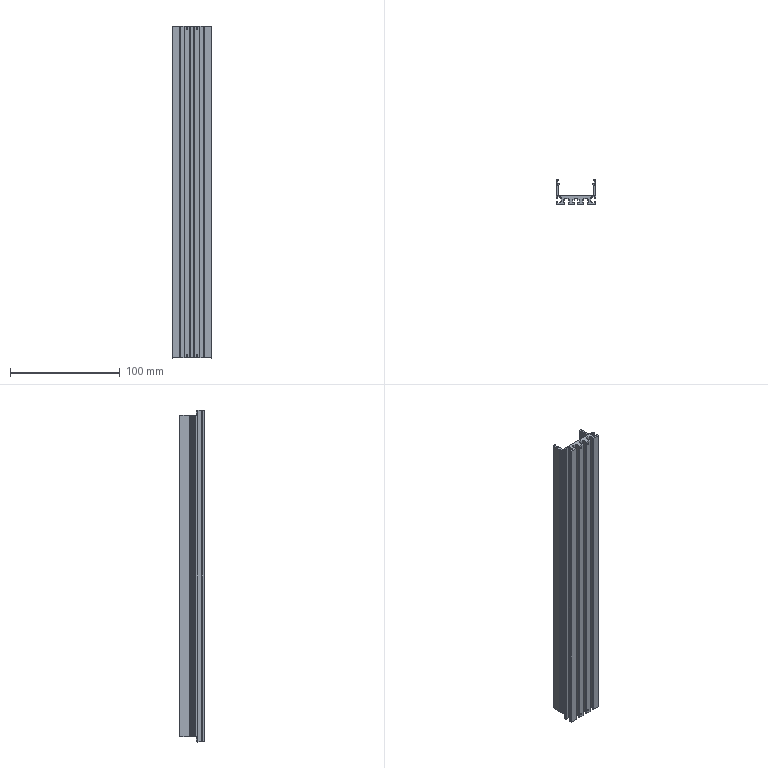Part | SolidWorks | features BaseBody 1 | 1 solid | 178 faces | box 36 x 22.6 x 302 mm | volume 68970 mm3 | plane 136 | cylinder 34 | cone 8 | commonest cylinder face diameters 0.6 x24 1.6 x8 2 x2